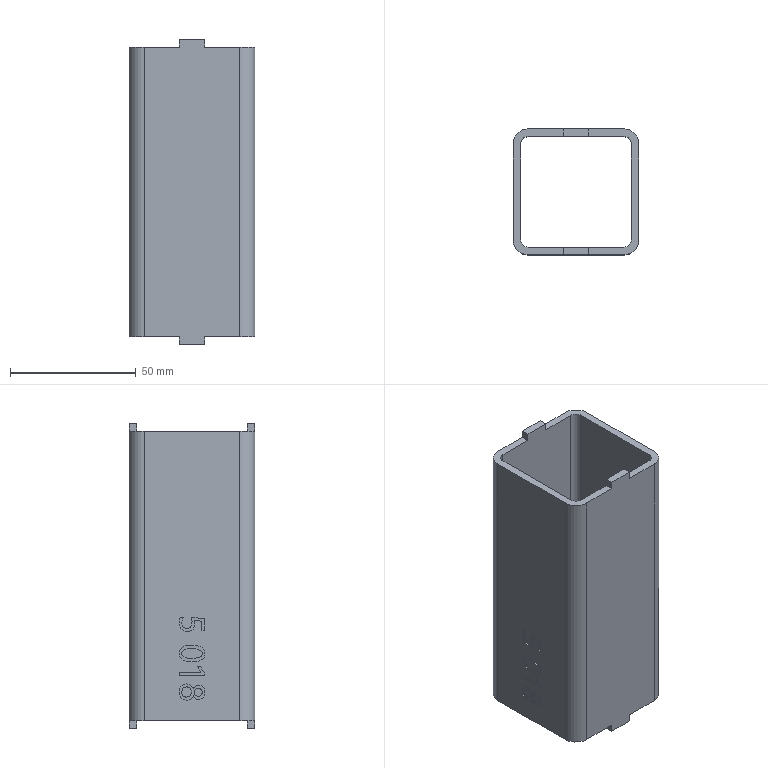Part | SolidWorks | features BaseBody 1 | 1 solid | 136 faces | box 50 x 50 x 121 mm | volume 62514 mm3 | spline 66 | plane 62 | cylinder 8 | commonest cylinder face diameters 6 x4 12 x4